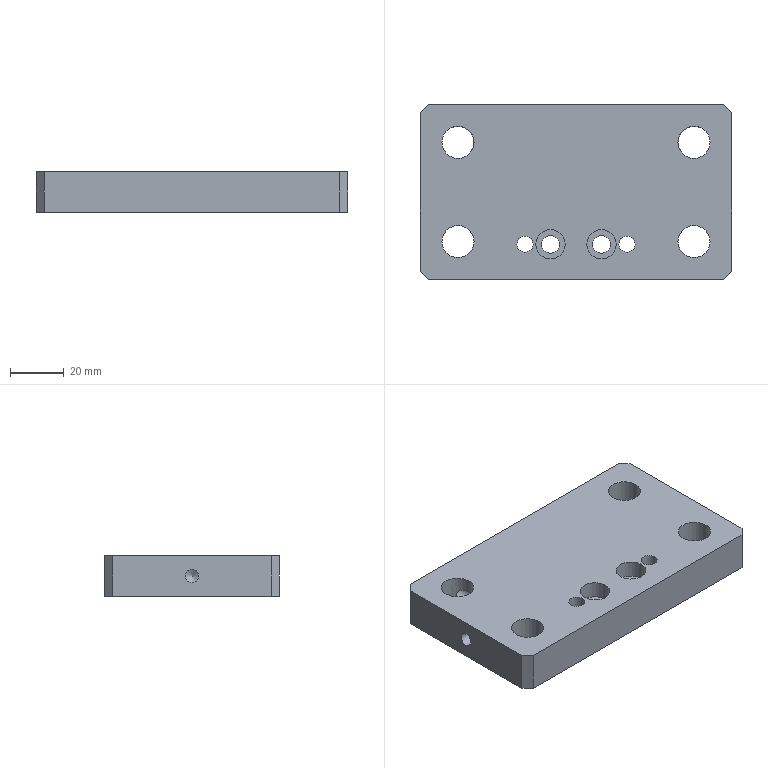Part | NX | features BREP 1 | 1 solid | 31 faces | box 116 x 65 x 15 mm | volume 102234 mm3 | cylinder 15 | plane 12 | cone 4 | commonest cylinder face diameters 5 x5 12 x4 6 x2 6.6 x2 11 x2
STEP:
#1=CARTESIAN_POINT('',(55.,-32.5,0.));
#2=VERTEX_POINT('',#1);
#3=CARTESIAN_POINT('',(58.,-29.5,0.));
#4=VERTEX_POINT('',#3);
#5=CARTESIAN_POINT('',(55.,-32.5,0.));
#6=DIRECTION('',(0.7071,0.7071,0.));
#7=VECTOR('',#6,1000.);
#8=LINE('',#5,#7);
#9=EDGE_CURVE('',#2,#4,#8,.T.);
#10=ORIENTED_EDGE('',*,*,#9,.F.);
#11=CARTESIAN_POINT('',(-55.,-32.5,0.));
#12=VERTEX_POINT('',#11);
#13=CARTESIAN_POINT('',(0.,-32.5,0.));
#14=DIRECTION('',(1.,0.,0.));
#15=VECTOR('',#14,1000.);
#16=LINE('',#13,#15);
#17=EDGE_CURVE('',#12,#2,#16,.T.);
#18=ORIENTED_EDGE('',*,*,#17,.F.);
#19=CARTESIAN_POINT('',(-58.,-29.5,0.));
#20=VERTEX_POINT('',#19);
#21=CARTESIAN_POINT('',(-58.,-29.5,0.));
#22=DIRECTION('',(0.7071,-0.7071,0.));
#23=VECTOR('',#22,1000.);
#24=LINE('',#21,#23);
#25=EDGE_CURVE('',#20,#12,#24,.T.);
#26=ORIENTED_EDGE('',*,*,#25,.F.);
#27=CARTESIAN_POINT('',(-58.,29.5,0.));
#28=VERTEX_POINT('',#27);
#29=CARTESIAN_POINT('',(-58.,0.,0.));
#30=DIRECTION('',(0.,-1.,0.));
#31=VECTOR('',#30,1000.);
#32=LINE('',#29,#31);
#33=EDGE_CURVE('',#28,#20,#32,.T.);
#34=ORIENTED_EDGE('',*,*,#33,.F.);
#35=CARTESIAN_POINT('',(-55.,32.5,0.));
#36=VERTEX_POINT('',#35);
#37=CARTESIAN_POINT('',(-55.,32.5,0.));
#38=DIRECTION('',(-0.7071,-0.7071,0.));
#39=VECTOR('',#38,1000.);
#40=LINE('',#37,#39);
#41=EDGE_CURVE('',#36,#28,#40,.T.);
#42=ORIENTED_EDGE('',*,*,#41,.F.);
#43=CARTESIAN_POINT('',(55.,32.5,0.));
#44=VERTEX_POINT('',#43);
#45=CARTESIAN_POINT('',(0.,32.5,0.));
#46=DIRECTION('',(-1.,0.,0.));
#47=VECTOR('',#46,1000.);
#48=LINE('',#45,#47);
#49=EDGE_CURVE('',#44,#36,#48,.T.);
#50=ORIENTED_EDGE('',*,*,#49,.F.);
#51=CARTESIAN_POINT('',(58.,29.5,0.));
#52=VERTEX_POINT('',#51);
#53=CARTESIAN_POINT('',(58.,29.5,0.));
#54=DIRECTION('',(-0.7071,0.7071,0.));
#55=VECTOR('',#54,1000.);
#56=LINE('',#53,#55);
#57=EDGE_CURVE('',#52,#44,#56,.T.);
#58=ORIENTED_EDGE('',*,*,#57,.F.);
#59=CARTESIAN_POINT('',(58.,0.,0.));
#60=DIRECTION('',(0.,1.,0.));
#61=VECTOR('',#60,1000.);
#62=LINE('',#59,#61);
#63=EDGE_CURVE('',#4,#52,#62,.T.);
#64=ORIENTED_EDGE('',*,*,#63,.F.);
#65=EDGE_LOOP('',(#10,#18,#26,#34,#42,#50,#58,#64));
#66=FACE_BOUND('',#65,.T.);
#67=CARTESIAN_POINT('',(38.,-18.5,0.));
#68=VERTEX_POINT('',#67);
#69=CARTESIAN_POINT('',(44.,-18.5,0.));
#70=DIRECTION('',(0.,0.,-1.));
#71=DIRECTION('',(-1.,0.,0.));
#72=AXIS2_PLACEMENT_3D('',#69,#70,#71);
#73=CIRCLE('',#72,6.);
#74=EDGE_CURVE('',#68,#68,#73,.T.);
#75=ORIENTED_EDGE('',*,*,#74,.F.);
#76=EDGE_LOOP('',(#75));
#77=FACE_BOUND('',#76,.T.);
#78=CARTESIAN_POINT('',(38.,18.5,0.));
#79=VERTEX_POINT('',#78);
#80=CARTESIAN_POINT('',(44.,18.5,0.));
#81=DIRECTION('',(0.,0.,-1.));
#82=DIRECTION('',(-1.,0.,0.));
#83=AXIS2_PLACEMENT_3D('',#80,#81,#82);
#84=CIRCLE('',#83,6.);
#85=EDGE_CURVE('',#79,#79,#84,.T.);
#86=ORIENTED_EDGE('',*,*,#85,.F.);
#87=EDGE_LOOP('',(#86));
#88=FACE_BOUND('',#87,.T.);
#89=CARTESIAN_POINT('',(-50.,18.5,0.));
#90=VERTEX_POINT('',#89);
#91=CARTESIAN_POINT('',(-44.,18.5,0.));
#92=DIRECTION('',(0.,0.,-1.));
#93=DIRECTION('',(-1.,0.,0.));
#94=AXIS2_PLACEMENT_3D('',#91,#92,#93);
#95=CIRCLE('',#94,6.);
#96=EDGE_CURVE('',#90,#90,#95,.T.);
#97=ORIENTED_EDGE('',*,*,#96,.F.);
#98=EDGE_LOOP('',(#97));
#99=FACE_BOUND('',#98,.T.);
#100=CARTESIAN_POINT('',(-50.,-18.5,0.));
#101=VERTEX_POINT('',#100);
#102=CARTESIAN_POINT('',(-44.,-18.5,0.));
#103=DIRECTION('',(0.,0.,-1.));
#104=DIRECTION('',(-1.,0.,0.));
#105=AXIS2_PLACEMENT_3D('',#102,#103,#104);
#106=CIRCLE('',#105,6.);
#107=EDGE_CURVE('',#101,#101,#106,.T.);
#108=ORIENTED_EDGE('',*,*,#107,.F.);
#109=EDGE_LOOP('',(#108));
#110=FACE_BOUND('',#109,.T.);
#111=CARTESIAN_POINT('',(16.,-19.5,0.));
#112=VERTEX_POINT('',#111);
#113=CARTESIAN_POINT('',(19.,-19.5,0.));
#114=DIRECTION('',(0.,0.,-1.));
#115=DIRECTION('',(-1.,0.,0.));
#116=AXIS2_PLACEMENT_3D('',#113,#114,#115);
#117=CIRCLE('',#116,3.);
#118=EDGE_CURVE('',#112,#112,#117,.T.);
#119=ORIENTED_EDGE('',*,*,#118,.F.);
#120=EDGE_LOOP('',(#119));
#121=FACE_BOUND('',#120,.T.);
#122=CARTESIAN_POINT('',(-22.,-19.5,0.));
#123=VERTEX_POINT('',#122);
#124=CARTESIAN_POINT('',(-19.,-19.5,0.));
#125=DIRECTION('',(0.,0.,-1.));
#126=DIRECTION('',(-1.,0.,0.));
#127=AXIS2_PLACEMENT_3D('',#124,#125,#126);
#128=CIRCLE('',#127,3.);
#129=EDGE_CURVE('',#123,#123,#128,.T.);
#130=ORIENTED_EDGE('',*,*,#129,.F.);
#131=EDGE_LOOP('',(#130));
#132=FACE_BOUND('',#131,.T.);
#133=CARTESIAN_POINT('',(12.8,-19.5,0.));
#134=VERTEX_POINT('',#133);
#135=CARTESIAN_POINT('',(9.5,-19.5,0.));
#136=DIRECTION('',(0.,0.,-1.));
#137=DIRECTION('',(1.,0.,0.));
#138=AXIS2_PLACEMENT_3D('',#135,#136,#137);
#139=CIRCLE('',#138,3.3);
#140=EDGE_CURVE('',#134,#134,#139,.T.);
#141=ORIENTED_EDGE('',*,*,#140,.F.);
#142=EDGE_LOOP('',(#141));
#143=FACE_BOUND('',#142,.T.);
#144=CARTESIAN_POINT('',(-6.2,-19.5,0.));
#145=VERTEX_POINT('',#144);
#146=CARTESIAN_POINT('',(-9.5,-19.5,0.));
#147=DIRECTION('',(0.,0.,-1.));
#148=DIRECTION('',(1.,0.,0.));
#149=AXIS2_PLACEMENT_3D('',#146,#147,#148);
#150=CIRCLE('',#149,3.3);
#151=EDGE_CURVE('',#145,#145,#150,.T.);
#152=ORIENTED_EDGE('',*,*,#151,.F.);
#153=EDGE_LOOP('',(#152));
#154=FACE_BOUND('',#153,.T.);
#155=CARTESIAN_POINT('',(0.,0.,0.));
#156=DIRECTION('',(0.,0.,1.));
#157=DIRECTION('',(-1.,0.,0.));
#158=AXIS2_PLACEMENT_3D('',#155,#156,#157);
#159=PLANE('',#158);
#160=ADVANCED_FACE('',(#66,#77,#88,#99,#110,#121,#132,#143,#154),#159,.F.);
#161=CARTESIAN_POINT('',(58.,-29.5,15.));
#162=VERTEX_POINT('',#161);
#163=CARTESIAN_POINT('',(58.,-29.5,15.));
#164=DIRECTION('',(0.,0.,1.));
#165=VECTOR('',#164,1000.);
#166=LINE('',#163,#165);
#167=EDGE_CURVE('',#4,#162,#166,.T.);
#168=ORIENTED_EDGE('',*,*,#167,.F.);
#169=ORIENTED_EDGE('',*,*,#63,.T.);
#170=CARTESIAN_POINT('',(58.,29.5,15.));
#171=VERTEX_POINT('',#170);
#172=CARTESIAN_POINT('',(58.,29.5,15.));
#173=DIRECTION('',(0.,0.,-1.));
#174=VECTOR('',#173,1000.);
#175=LINE('',#172,#174);
#176=EDGE_CURVE('',#171,#52,#175,.T.);
#177=ORIENTED_EDGE('',*,*,#176,.F.);
#178=CARTESIAN_POINT('',(58.,32.5,15.));
#179=DIRECTION('',(0.,1.,0.));
#180=VECTOR('',#179,1000.);
#181=LINE('',#178,#180);
#182=EDGE_CURVE('',#162,#171,#181,.T.);
#183=ORIENTED_EDGE('',*,*,#182,.F.);
#184=EDGE_LOOP('',(#168,#169,#177,#183));
#185=FACE_BOUND('',#184,.T.);
#186=CARTESIAN_POINT('',(58.,0.,5.));
#187=VERTEX_POINT('',#186);
#188=CARTESIAN_POINT('',(58.,0.,7.5));
#189=DIRECTION('',(1.,0.,0.));
#190=DIRECTION('',(0.,0.,-1.));
#191=AXIS2_PLACEMENT_3D('',#188,#189,#190);
#192=CIRCLE('',#191,2.5);
#193=EDGE_CURVE('',#187,#187,#192,.T.);
#194=ORIENTED_EDGE('',*,*,#193,.F.);
#195=EDGE_LOOP('',(#194));
#196=FACE_BOUND('',#195,.T.);
#197=CARTESIAN_POINT('',(58.,32.5,15.));
#198=DIRECTION('',(-1.,0.,0.));
#199=DIRECTION('',(0.,1.,0.));
#200=AXIS2_PLACEMENT_3D('',#197,#198,#199);
#201=PLANE('',#200);
#202=ADVANCED_FACE('',(#185,#196),#201,.F.);
#203=CARTESIAN_POINT('',(55.,-32.5,15.));
#204=VERTEX_POINT('',#203);
#205=CARTESIAN_POINT('',(55.,-32.5,15.));
#206=DIRECTION('',(0.,0.,1.));
#207=VECTOR('',#206,1000.);
#208=LINE('',#205,#207);
#209=EDGE_CURVE('',#2,#204,#208,.T.);
#210=ORIENTED_EDGE('',*,*,#209,.F.);
#211=ORIENTED_EDGE('',*,*,#9,.T.);
#212=ORIENTED_EDGE('',*,*,#167,.T.);
#213=CARTESIAN_POINT('',(58.,-29.5,15.));
#214=DIRECTION('',(0.7071,0.7071,0.));
#215=VECTOR('',#214,1000.);
#216=LINE('',#213,#215);
#217=EDGE_CURVE('',#204,#162,#216,.T.);
#218=ORIENTED_EDGE('',*,*,#217,.F.);
#219=EDGE_LOOP('',(#210,#211,#212,#218));
#220=FACE_BOUND('',#219,.T.);
#221=CARTESIAN_POINT('',(58.,-29.5,15.));
#222=DIRECTION('',(-0.7071,0.7071,0.));
#223=DIRECTION('',(0.7071,0.7071,0.));
#224=AXIS2_PLACEMENT_3D('',#221,#222,#223);
#225=PLANE('',#224);
#226=ADVANCED_FACE('',(#220),#225,.F.);
#227=ORIENTED_EDGE('',*,*,#209,.T.);
#228=CARTESIAN_POINT('',(-55.,-32.5,15.));
#229=VERTEX_POINT('',#228);
#230=CARTESIAN_POINT('',(-58.,-32.5,15.));
#231=DIRECTION('',(1.,0.,0.));
#232=VECTOR('',#231,1000.);
#233=LINE('',#230,#232);
#234=EDGE_CURVE('',#229,#204,#233,.T.);
#235=ORIENTED_EDGE('',*,*,#234,.F.);
#236=CARTESIAN_POINT('',(-55.,-32.5,15.));
#237=DIRECTION('',(0.,0.,1.));
#238=VECTOR('',#237,1000.);
#239=LINE('',#236,#238);
#240=EDGE_CURVE('',#12,#229,#239,.T.);
#241=ORIENTED_EDGE('',*,*,#240,.F.);
#242=ORIENTED_EDGE('',*,*,#17,.T.);
#243=EDGE_LOOP('',(#227,#235,#241,#242));
#244=FACE_BOUND('',#243,.T.);
#245=CARTESIAN_POINT('',(-58.,-32.5,15.));
#246=DIRECTION('',(0.,1.,0.));
#247=DIRECTION('',(0.,0.,-1.));
#248=AXIS2_PLACEMENT_3D('',#245,#246,#247);
#249=PLANE('',#248);
#250=ADVANCED_FACE('',(#244),#249,.F.);
#251=CARTESIAN_POINT('',(-58.,-29.5,15.));
#252=VERTEX_POINT('',#251);
#253=CARTESIAN_POINT('',(-58.,-29.5,15.));
#254=DIRECTION('',(0.,0.,1.));
#255=VECTOR('',#254,1000.);
#256=LINE('',#253,#255);
#257=EDGE_CURVE('',#20,#252,#256,.T.);
#258=ORIENTED_EDGE('',*,*,#257,.F.);
#259=ORIENTED_EDGE('',*,*,#25,.T.);
#260=ORIENTED_EDGE('',*,*,#240,.T.);
#261=CARTESIAN_POINT('',(-55.,-32.5,15.));
#262=DIRECTION('',(0.7071,-0.7071,0.));
#263=VECTOR('',#262,1000.);
#264=LINE('',#261,#263);
#265=EDGE_CURVE('',#252,#229,#264,.T.);
#266=ORIENTED_EDGE('',*,*,#265,.F.);
#267=EDGE_LOOP('',(#258,#259,#260,#266));
#268=FACE_BOUND('',#267,.T.);
#269=CARTESIAN_POINT('',(-55.,-32.5,15.));
#270=DIRECTION('',(0.7071,0.7071,0.));
#271=DIRECTION('',(0.7071,-0.7071,0.));
#272=AXIS2_PLACEMENT_3D('',#269,#270,#271);
#273=PLANE('',#272);
#274=ADVANCED_FACE('',(#268),#273,.F.);
#275=ORIENTED_EDGE('',*,*,#257,.T.);
#276=CARTESIAN_POINT('',(-58.,29.5,15.));
#277=VERTEX_POINT('',#276);
#278=CARTESIAN_POINT('',(-58.,32.5,15.));
#279=DIRECTION('',(0.,-1.,0.));
#280=VECTOR('',#279,1000.);
#281=LINE('',#278,#280);
#282=EDGE_CURVE('',#277,#252,#281,.T.);
#283=ORIENTED_EDGE('',*,*,#282,.F.);
#284=CARTESIAN_POINT('',(-58.,29.5,15.));
#285=DIRECTION('',(0.,0.,1.));
#286=VECTOR('',#285,1000.);
#287=LINE('',#284,#286);
#288=EDGE_CURVE('',#28,#277,#287,.T.);
#289=ORIENTED_EDGE('',*,*,#288,.F.);
#290=ORIENTED_EDGE('',*,*,#33,.T.);
#291=EDGE_LOOP('',(#275,#283,#289,#290));
#292=FACE_BOUND('',#291,.T.);
#293=CARTESIAN_POINT('',(-58.,0.,10.));
#294=VERTEX_POINT('',#293);
#295=CARTESIAN_POINT('',(-58.,0.,7.5));
#296=DIRECTION('',(-1.,0.,0.));
#297=DIRECTION('',(0.,0.,1.));
#298=AXIS2_PLACEMENT_3D('',#295,#296,#297);
#299=CIRCLE('',#298,2.5);
#300=EDGE_CURVE('',#294,#294,#299,.T.);
#301=ORIENTED_EDGE('',*,*,#300,.F.);
#302=EDGE_LOOP('',(#301));
#303=FACE_BOUND('',#302,.T.);
#304=CARTESIAN_POINT('',(-58.,32.5,15.));
#305=DIRECTION('',(1.,0.,0.));
#306=DIRECTION('',(0.,-1.,0.));
#307=AXIS2_PLACEMENT_3D('',#304,#305,#306);
#308=PLANE('',#307);
#309=ADVANCED_FACE('',(#292,#303),#308,.F.);
#310=CARTESIAN_POINT('',(-55.,32.5,15.));
#311=VERTEX_POINT('',#310);
#312=CARTESIAN_POINT('',(-55.,32.5,15.));
#313=DIRECTION('',(0.,0.,1.));
#314=VECTOR('',#313,1000.);
#315=LINE('',#312,#314);
#316=EDGE_CURVE('',#36,#311,#315,.T.);
#317=ORIENTED_EDGE('',*,*,#316,.F.);
#318=ORIENTED_EDGE('',*,*,#41,.T.);
#319=ORIENTED_EDGE('',*,*,#288,.T.);
#320=CARTESIAN_POINT('',(-58.,29.5,15.));
#321=DIRECTION('',(-0.7071,-0.7071,0.));
#322=VECTOR('',#321,1000.);
#323=LINE('',#320,#322);
#324=EDGE_CURVE('',#311,#277,#323,.T.);
#325=ORIENTED_EDGE('',*,*,#324,.F.);
#326=EDGE_LOOP('',(#317,#318,#319,#325));
#327=FACE_BOUND('',#326,.T.);
#328=CARTESIAN_POINT('',(-58.,29.5,15.));
#329=DIRECTION('',(0.7071,-0.7071,0.));
#330=DIRECTION('',(-0.7071,-0.7071,0.));
#331=AXIS2_PLACEMENT_3D('',#328,#329,#330);
#332=PLANE('',#331);
#333=ADVANCED_FACE('',(#327),#332,.F.);
#334=CARTESIAN_POINT('',(55.,32.5,15.));
#335=VERTEX_POINT('',#334);
#336=CARTESIAN_POINT('',(55.,32.5,15.));
#337=DIRECTION('',(0.,0.,1.));
#338=VECTOR('',#337,1000.);
#339=LINE('',#336,#338);
#340=EDGE_CURVE('',#44,#335,#339,.T.);
#341=ORIENTED_EDGE('',*,*,#340,.F.);
#342=ORIENTED_EDGE('',*,*,#49,.T.);
#343=ORIENTED_EDGE('',*,*,#316,.T.);
#344=CARTESIAN_POINT('',(-58.,32.5,15.));
#345=DIRECTION('',(-1.,0.,0.));
#346=VECTOR('',#345,1000.);
#347=LINE('',#344,#346);
#348=EDGE_CURVE('',#335,#311,#347,.T.);
#349=ORIENTED_EDGE('',*,*,#348,.F.);
#350=EDGE_LOOP('',(#341,#342,#343,#349));
#351=FACE_BOUND('',#350,.T.);
#352=CARTESIAN_POINT('',(37.5,32.5,10.));
#353=VERTEX_POINT('',#352);
#354=CARTESIAN_POINT('',(37.5,32.5,7.5));
#355=DIRECTION('',(0.,1.,0.));
#356=DIRECTION('',(0.,0.,1.));
#357=AXIS2_PLACEMENT_3D('',#354,#355,#356);
#358=CIRCLE('',#357,2.5);
#359=EDGE_CURVE('',#353,#353,#358,.T.);
#360=ORIENTED_EDGE('',*,*,#359,.F.);
#361=EDGE_LOOP('',(#360));
#362=FACE_BOUND('',#361,.T.);
#363=CARTESIAN_POINT('',(-37.5,32.5,10.));
#364=VERTEX_POINT('',#363);
#365=CARTESIAN_POINT('',(-37.5,32.5,7.5));
#366=DIRECTION('',(0.,1.,0.));
#367=DIRECTION('',(0.,0.,1.));
#368=AXIS2_PLACEMENT_3D('',#365,#366,#367);
#369=CIRCLE('',#368,2.5);
#370=EDGE_CURVE('',#364,#364,#369,.T.);
#371=ORIENTED_EDGE('',*,*,#370,.F.);
#372=EDGE_LOOP('',(#371));
#373=FACE_BOUND('',#372,.T.);
#374=CARTESIAN_POINT('',(-58.,32.5,15.));
#375=DIRECTION('',(0.,-1.,0.));
#376=DIRECTION('',(0.,0.,1.));
#377=AXIS2_PLACEMENT_3D('',#374,#375,#376);
#378=PLANE('',#377);
#379=ADVANCED_FACE('',(#351,#362,#373),#378,.F.);
#380=ORIENTED_EDGE('',*,*,#176,.T.);
#381=ORIENTED_EDGE('',*,*,#57,.T.);
#382=ORIENTED_EDGE('',*,*,#340,.T.);
#383=CARTESIAN_POINT('',(55.,32.5,15.));
#384=DIRECTION('',(-0.7071,0.7071,0.));
#385=VECTOR('',#384,1000.);
#386=LINE('',#383,#385);
#387=EDGE_CURVE('',#171,#335,#386,.T.);
#388=ORIENTED_EDGE('',*,*,#387,.F.);
#389=EDGE_LOOP('',(#380,#381,#382,#388));
#390=FACE_BOUND('',#389,.T.);
#391=CARTESIAN_POINT('',(55.,32.5,15.));
#392=DIRECTION('',(-0.7071,-0.7071,0.));
#393=DIRECTION('',(-0.7071,0.7071,0.));
#394=AXIS2_PLACEMENT_3D('',#391,#392,#393);
#395=PLANE('',#394);
#396=ADVANCED_FACE('',(#390),#395,.F.);
#397=CARTESIAN_POINT('',(38.,-18.5,15.));
#398=VERTEX_POINT('',#397);
#399=CARTESIAN_POINT('',(44.,-18.5,15.));
#400=DIRECTION('',(0.,0.,-1.));
#401=DIRECTION('',(-1.,0.,0.));
#402=AXIS2_PLACEMENT_3D('',#399,#400,#401);
#403=CIRCLE('',#402,6.);
#404=EDGE_CURVE('',#398,#398,#403,.T.);
#405=ORIENTED_EDGE('',*,*,#404,.F.);
#406=EDGE_LOOP('',(#405));
#407=FACE_BOUND('',#406,.T.);
#408=ORIENTED_EDGE('',*,*,#74,.T.);
#409=EDGE_LOOP('',(#408));
#410=FACE_BOUND('',#409,.T.);
#411=CARTESIAN_POINT('',(44.,-18.5,0.));
#412=DIRECTION('',(0.,0.,-1.));
#413=DIRECTION('',(1.,0.,0.));
#414=AXIS2_PLACEMENT_3D('',#411,#412,#413);
#415=CYLINDRICAL_SURFACE('',#414,6.);
#416=ADVANCED_FACE('',(#407,#410),#415,.F.);
#417=CARTESIAN_POINT('',(38.084,17.5,5.069));
#418=VERTEX_POINT('',#417);
#419=CARTESIAN_POINT('',(38.084,17.5,9.931));
#420=VERTEX_POINT('',#419);
#421=CARTESIAN_POINT('',(38.084,17.5,5.069));
#422=CARTESIAN_POINT('',(37.983,18.098,5.045));
#423=CARTESIAN_POINT('',(37.966,19.305,5.043));
#424=CARTESIAN_POINT('',(38.461,21.047,5.154));
#425=CARTESIAN_POINT('',(39.481,22.542,5.725));
#426=CARTESIAN_POINT('',(40.257,23.185,7.487));
#427=CARTESIAN_POINT('',(39.492,22.553,9.265));
#428=CARTESIAN_POINT('',(38.471,21.068,9.843));
#429=CARTESIAN_POINT('',(37.966,19.32,9.957));
#430=CARTESIAN_POINT('',(37.983,18.098,9.955));
#431=CARTESIAN_POINT('',(38.084,17.5,9.931));
#432=B_SPLINE_CURVE_WITH_KNOTS('',3,(#421,#422,#423,#424,#425,#426,#427,#428,#429,#430,#431),.UNSPECIFIED.,.F.,.F.,(4,1,1,1,1,1,1,1,4),(0.,0.001794,0.003588,0.005381,0.007175,0.008969,0.01076,0.01256,0.01435),.UNSPECIFIED.);
#433=EDGE_CURVE('',#418,#420,#432,.T.);
#434=ORIENTED_EDGE('',*,*,#433,.F.);
#435=CARTESIAN_POINT('',(38.084,17.5,9.931));
#436=CARTESIAN_POINT('',(38.121,17.28,9.545));
#437=CARTESIAN_POINT('',(38.219,16.853,8.787));
#438=CARTESIAN_POINT('',(38.404,16.329,7.497));
#439=CARTESIAN_POINT('',(38.218,16.855,6.211));
#440=CARTESIAN_POINT('',(38.121,17.281,5.454));
#441=CARTESIAN_POINT('',(38.084,17.5,5.069));
#442=B_SPLINE_CURVE_WITH_KNOTS('',3,(#435,#436,#437,#438,#439,#440,#441),.UNSPECIFIED.,.F.,.F.,(4,1,1,1,4),(0.,0.001335,0.002669,0.004004,0.005339),.UNSPECIFIED.);
#443=EDGE_CURVE('',#420,#418,#442,.T.);
#444=ORIENTED_EDGE('',*,*,#443,.F.);
#445=EDGE_LOOP('',(#434,#444));
#446=FACE_BOUND('',#445,.T.);
#447=CARTESIAN_POINT('',(38.,18.5,15.));
#448=VERTEX_POINT('',#447);
#449=CARTESIAN_POINT('',(44.,18.5,15.));
#450=DIRECTION('',(0.,0.,-1.));
#451=DIRECTION('',(-1.,0.,0.));
#452=AXIS2_PLACEMENT_3D('',#449,#450,#451);
#453=CIRCLE('',#452,6.);
#454=EDGE_CURVE('',#448,#448,#453,.T.);
#455=ORIENTED_EDGE('',*,*,#454,.F.);
#456=EDGE_LOOP('',(#455));
#457=FACE_BOUND('',#456,.T.);
#458=ORIENTED_EDGE('',*,*,#85,.T.);
#459=EDGE_LOOP('',(#458));
#460=FACE_BOUND('',#459,.T.);
#461=CARTESIAN_POINT('',(44.,18.5,0.));
#462=DIRECTION('',(0.,0.,-1.));
#463=DIRECTION('',(1.,0.,0.));
#464=AXIS2_PLACEMENT_3D('',#461,#462,#463);
#465=CYLINDRICAL_SURFACE('',#464,6.);
#466=ADVANCED_FACE('',(#446,#457,#460),#465,.F.);
#467=ORIENTED_EDGE('',*,*,#96,.T.);
#468=EDGE_LOOP('',(#467));
#469=FACE_BOUND('',#468,.T.);
#470=CARTESIAN_POINT('',(-50.,18.5,15.));
#471=VERTEX_POINT('',#470);
#472=CARTESIAN_POINT('',(-44.,18.5,15.));
#473=DIRECTION('',(0.,0.,-1.));
#474=DIRECTION('',(-1.,0.,0.));
#475=AXIS2_PLACEMENT_3D('',#472,#473,#474);
#476=CIRCLE('',#475,6.);
#477=EDGE_CURVE('',#471,#471,#476,.T.);
#478=ORIENTED_EDGE('',*,*,#477,.F.);
#479=EDGE_LOOP('',(#478));
#480=FACE_BOUND('',#479,.T.);
#481=CARTESIAN_POINT('',(-38.084,17.5,5.069));
#482=VERTEX_POINT('',#481);
#483=CARTESIAN_POINT('',(-38.084,17.5,9.931));
#484=VERTEX_POINT('',#483);
#485=CARTESIAN_POINT('',(-38.084,17.5,5.069));
#486=CARTESIAN_POINT('',(-38.121,17.28,5.455));
#487=CARTESIAN_POINT('',(-38.219,16.853,6.213));
#488=CARTESIAN_POINT('',(-38.404,16.329,7.503));
#489=CARTESIAN_POINT('',(-38.218,16.855,8.789));
#490=CARTESIAN_POINT('',(-38.121,17.281,9.546));
#491=CARTESIAN_POINT('',(-38.084,17.5,9.931));
#492=B_SPLINE_CURVE_WITH_KNOTS('',3,(#485,#486,#487,#488,#489,#490,#491),.UNSPECIFIED.,.F.,.F.,(4,1,1,1,4),(0.,0.001335,0.002669,0.004004,0.005339),.UNSPECIFIED.);
#493=EDGE_CURVE('',#482,#484,#492,.T.);
#494=ORIENTED_EDGE('',*,*,#493,.F.);
#495=CARTESIAN_POINT('',(-38.084,17.5,9.931));
#496=CARTESIAN_POINT('',(-37.983,18.098,9.955));
#497=CARTESIAN_POINT('',(-37.966,19.305,9.957));
#498=CARTESIAN_POINT('',(-38.461,21.047,9.846));
#499=CARTESIAN_POINT('',(-39.481,22.542,9.275));
#500=CARTESIAN_POINT('',(-40.257,23.185,7.513));
#501=CARTESIAN_POINT('',(-39.492,22.553,5.735));
#502=CARTESIAN_POINT('',(-38.471,21.068,5.157));
#503=CARTESIAN_POINT('',(-37.966,19.32,5.043));
#504=CARTESIAN_POINT('',(-37.983,18.098,5.045));
#505=CARTESIAN_POINT('',(-38.084,17.5,5.069));
#506=B_SPLINE_CURVE_WITH_KNOTS('',3,(#495,#496,#497,#498,#499,#500,#501,#502,#503,#504,#505),.UNSPECIFIED.,.F.,.F.,(4,1,1,1,1,1,1,1,4),(0.,0.001794,0.003588,0.005381,0.007175,0.008969,0.01076,0.01256,0.01435),.UNSPECIFIED.);
#507=EDGE_CURVE('',#484,#482,#506,.T.);
#508=ORIENTED_EDGE('',*,*,#507,.F.);
#509=EDGE_LOOP('',(#494,#508));
#510=FACE_BOUND('',#509,.T.);
#511=CARTESIAN_POINT('',(-44.,18.5,0.));
#512=DIRECTION('',(0.,0.,-1.));
#513=DIRECTION('',(1.,0.,0.));
#514=AXIS2_PLACEMENT_3D('',#511,#512,#513);
#515=CYLINDRICAL_SURFACE('',#514,6.);
#516=ADVANCED_FACE('',(#469,#480,#510),#515,.F.);
#517=CARTESIAN_POINT('',(-50.,-18.5,15.));
#518=VERTEX_POINT('',#517);
#519=CARTESIAN_POINT('',(-44.,-18.5,15.));
#520=DIRECTION('',(0.,0.,-1.));
#521=DIRECTION('',(-1.,0.,0.));
#522=AXIS2_PLACEMENT_3D('',#519,#520,#521);
#523=CIRCLE('',#522,6.);
#524=EDGE_CURVE('',#518,#518,#523,.T.);
#525=ORIENTED_EDGE('',*,*,#524,.F.);
#526=EDGE_LOOP('',(#525));
#527=FACE_BOUND('',#526,.T.);
#528=ORIENTED_EDGE('',*,*,#107,.T.);
#529=EDGE_LOOP('',(#528));
#530=FACE_BOUND('',#529,.T.);
#531=CARTESIAN_POINT('',(-44.,-18.5,0.));
#532=DIRECTION('',(0.,0.,-1.));
#533=DIRECTION('',(1.,0.,0.));
#534=AXIS2_PLACEMENT_3D('',#531,#532,#533);
#535=CYLINDRICAL_SURFACE('',#534,6.);
#536=ADVANCED_FACE('',(#527,#530),#535,.F.);
#537=CARTESIAN_POINT('',(16.,-19.5,15.));
#538=VERTEX_POINT('',#537);
#539=CARTESIAN_POINT('',(19.,-19.5,15.));
#540=DIRECTION('',(0.,0.,-1.));
#541=DIRECTION('',(-1.,0.,0.));
#542=AXIS2_PLACEMENT_3D('',#539,#540,#541);
#543=CIRCLE('',#542,3.);
#544=EDGE_CURVE('',#538,#538,#543,.T.);
#545=ORIENTED_EDGE('',*,*,#544,.F.);
#546=EDGE_LOOP('',(#545));
#547=FACE_BOUND('',#546,.T.);
#548=ORIENTED_EDGE('',*,*,#118,.T.);
#549=EDGE_LOOP('',(#548));
#550=FACE_BOUND('',#549,.T.);
#551=CARTESIAN_POINT('',(19.,-19.5,0.));
#552=DIRECTION('',(0.,0.,-1.));
#553=DIRECTION('',(1.,0.,0.));
#554=AXIS2_PLACEMENT_3D('',#551,#552,#553);
#555=CYLINDRICAL_SURFACE('',#554,3.);
#556=ADVANCED_FACE('',(#547,#550),#555,.F.);
#557=CARTESIAN_POINT('',(-22.,-19.5,15.));
#558=VERTEX_POINT('',#557);
#559=CARTESIAN_POINT('',(-19.,-19.5,15.));
#560=DIRECTION('',(0.,0.,-1.));
#561=DIRECTION('',(-1.,0.,0.));
#562=AXIS2_PLACEMENT_3D('',#559,#560,#561);
#563=CIRCLE('',#562,3.);
#564=EDGE_CURVE('',#558,#558,#563,.T.);
#565=ORIENTED_EDGE('',*,*,#564,.F.);
#566=EDGE_LOOP('',(#565));
#567=FACE_BOUND('',#566,.T.);
#568=ORIENTED_EDGE('',*,*,#129,.T.);
#569=EDGE_LOOP('',(#568));
#570=FACE_BOUND('',#569,.T.);
#571=CARTESIAN_POINT('',(-19.,-19.5,0.));
#572=DIRECTION('',(0.,0.,-1.));
#573=DIRECTION('',(1.,0.,0.));
#574=AXIS2_PLACEMENT_3D('',#571,#572,#573);
#575=CYLINDRICAL_SURFACE('',#574,3.);
#576=ADVANCED_FACE('',(#567,#570),#575,.F.);
#577=ORIENTED_EDGE('',*,*,#140,.T.);
#578=EDGE_LOOP('',(#577));
#579=FACE_BOUND('',#578,.T.);
#580=CARTESIAN_POINT('',(12.8,-19.5,8.6));
#581=VERTEX_POINT('',#580);
#582=CARTESIAN_POINT('',(9.5,-19.5,8.6));
#583=DIRECTION('',(0.,0.,-1.));
#584=DIRECTION('',(1.,0.,0.));
#585=AXIS2_PLACEMENT_3D('',#582,#583,#584);
#586=CIRCLE('',#585,3.3);
#587=EDGE_CURVE('',#581,#581,#586,.T.);
#588=ORIENTED_EDGE('',*,*,#587,.F.);
#589=EDGE_LOOP('',(#588));
#590=FACE_BOUND('',#589,.T.);
#591=CARTESIAN_POINT('',(9.5,-19.5,15.));
#592=DIRECTION('',(0.,0.,1.));
#593=DIRECTION('',(-1.,0.,0.));
#594=AXIS2_PLACEMENT_3D('',#591,#592,#593);
#595=CYLINDRICAL_SURFACE('',#594,3.3);
#596=ADVANCED_FACE('',(#579,#590),#595,.F.);
#597=ORIENTED_EDGE('',*,*,#151,.T.);
#598=EDGE_LOOP('',(#597));
#599=FACE_BOUND('',#598,.T.);
#600=CARTESIAN_POINT('',(-6.2,-19.5,8.6));
#601=VERTEX_POINT('',#600);
#602=CARTESIAN_POINT('',(-9.5,-19.5,8.6));
#603=DIRECTION('',(0.,0.,-1.));
#604=DIRECTION('',(1.,0.,0.));
#605=AXIS2_PLACEMENT_3D('',#602,#603,#604);
#606=CIRCLE('',#605,3.3);
#607=EDGE_CURVE('',#601,#601,#606,.T.);
#608=ORIENTED_EDGE('',*,*,#607,.F.);
#609=EDGE_LOOP('',(#608));
#610=FACE_BOUND('',#609,.T.);
#611=CARTESIAN_POINT('',(-9.5,-19.5,15.));
#612=DIRECTION('',(0.,0.,1.));
#613=DIRECTION('',(-1.,0.,0.));
#614=AXIS2_PLACEMENT_3D('',#611,#612,#613);
#615=CYLINDRICAL_SURFACE('',#614,3.3);
#616=ADVANCED_FACE('',(#599,#610),#615,.F.);
#617=ORIENTED_EDGE('',*,*,#282,.T.);
#618=ORIENTED_EDGE('',*,*,#265,.T.);
#619=ORIENTED_EDGE('',*,*,#234,.T.);
#620=ORIENTED_EDGE('',*,*,#217,.T.);
#621=ORIENTED_EDGE('',*,*,#182,.T.);
#622=ORIENTED_EDGE('',*,*,#387,.T.);
#623=ORIENTED_EDGE('',*,*,#348,.T.);
#624=ORIENTED_EDGE('',*,*,#324,.T.);
#625=EDGE_LOOP('',(#617,#618,#619,#620,#621,#622,#623,#624));
#626=FACE_BOUND('',#625,.T.);
#627=ORIENTED_EDGE('',*,*,#404,.T.);
#628=EDGE_LOOP('',(#627));
#629=FACE_BOUND('',#628,.T.);
#630=ORIENTED_EDGE('',*,*,#454,.T.);
#631=EDGE_LOOP('',(#630));
#632=FACE_BOUND('',#631,.T.);
#633=ORIENTED_EDGE('',*,*,#477,.T.);
#634=EDGE_LOOP('',(#633));
#635=FACE_BOUND('',#634,.T.);
#636=ORIENTED_EDGE('',*,*,#524,.T.);
#637=EDGE_LOOP('',(#636));
#638=FACE_BOUND('',#637,.T.);
#639=ORIENTED_EDGE('',*,*,#544,.T.);
#640=EDGE_LOOP('',(#639));
#641=FACE_BOUND('',#640,.T.);
#642=ORIENTED_EDGE('',*,*,#564,.T.);
#643=EDGE_LOOP('',(#642));
#644=FACE_BOUND('',#643,.T.);
#645=CARTESIAN_POINT('',(15.,-19.5,15.));
#646=VERTEX_POINT('',#645);
#647=CARTESIAN_POINT('',(9.5,-19.5,15.));
#648=DIRECTION('',(0.,0.,-1.));
#649=DIRECTION('',(1.,0.,0.));
#650=AXIS2_PLACEMENT_3D('',#647,#648,#649);
#651=CIRCLE('',#650,5.5);
#652=EDGE_CURVE('',#646,#646,#651,.T.);
#653=ORIENTED_EDGE('',*,*,#652,.T.);
#654=EDGE_LOOP('',(#653));
#655=FACE_BOUND('',#654,.T.);
#656=CARTESIAN_POINT('',(-4.,-19.5,15.));
#657=VERTEX_POINT('',#656);
#658=CARTESIAN_POINT('',(-9.5,-19.5,15.));
#659=DIRECTION('',(0.,0.,-1.));
#660=DIRECTION('',(1.,0.,0.));
#661=AXIS2_PLACEMENT_3D('',#658,#659,#660);
#662=CIRCLE('',#661,5.5);
#663=EDGE_CURVE('',#657,#657,#662,.T.);
#664=ORIENTED_EDGE('',*,*,#663,.T.);
#665=EDGE_LOOP('',(#664));
#666=FACE_BOUND('',#665,.T.);
#667=CARTESIAN_POINT('',(0.,0.,15.));
#668=DIRECTION('',(0.,0.,1.));
#669=DIRECTION('',(-1.,0.,0.));
#670=AXIS2_PLACEMENT_3D('',#667,#668,#669);
#671=PLANE('',#670);
#672=ADVANCED_FACE('',(#626,#629,#632,#635,#638,#641,#644,#655,#666),#671,.T.);
#673=CARTESIAN_POINT('',(43.,0.,5.));
#674=VERTEX_POINT('',#673);
#675=CARTESIAN_POINT('',(43.,0.,7.5));
#676=DIRECTION('',(1.,0.,0.));
#677=DIRECTION('',(0.,0.,-1.));
#678=AXIS2_PLACEMENT_3D('',#675,#676,#677);
#679=CIRCLE('',#678,2.5);
#680=EDGE_CURVE('',#674,#674,#679,.T.);
#681=ORIENTED_EDGE('',*,*,#680,.F.);
#682=EDGE_LOOP('',(#681));
#683=FACE_BOUND('',#682,.T.);
#684=ORIENTED_EDGE('',*,*,#193,.T.);
#685=EDGE_LOOP('',(#684));
#686=FACE_BOUND('',#685,.T.);
#687=CARTESIAN_POINT('',(58.,0.,7.5));
#688=DIRECTION('',(1.,0.,0.));
#689=DIRECTION('',(0.,0.,1.));
#690=AXIS2_PLACEMENT_3D('',#687,#688,#689);
#691=CYLINDRICAL_SURFACE('',#690,2.5);
#692=ADVANCED_FACE('',(#683,#686),#691,.F.);
#693=CARTESIAN_POINT('',(-43.,0.,10.));
#694=VERTEX_POINT('',#693);
#695=CARTESIAN_POINT('',(-43.,0.,7.5));
#696=DIRECTION('',(-1.,0.,0.));
#697=DIRECTION('',(0.,0.,1.));
#698=AXIS2_PLACEMENT_3D('',#695,#696,#697);
#699=CIRCLE('',#698,2.5);
#700=EDGE_CURVE('',#694,#694,#699,.T.);
#701=ORIENTED_EDGE('',*,*,#700,.F.);
#702=EDGE_LOOP('',(#701));
#703=FACE_BOUND('',#702,.T.);
#704=ORIENTED_EDGE('',*,*,#300,.T.);
#705=EDGE_LOOP('',(#704));
#706=FACE_BOUND('',#705,.T.);
#707=CARTESIAN_POINT('',(-58.,0.,7.5));
#708=DIRECTION('',(-1.,0.,0.));
#709=DIRECTION('',(0.,0.,-1.));
#710=AXIS2_PLACEMENT_3D('',#707,#708,#709);
#711=CYLINDRICAL_SURFACE('',#710,2.5);
#712=ADVANCED_FACE('',(#703,#706),#711,.F.);
#713=ORIENTED_EDGE('',*,*,#433,.T.);
#714=CARTESIAN_POINT('',(37.5,17.5,7.5));
#715=DIRECTION('',(0.,1.,0.));
#716=DIRECTION('',(0.,0.,1.));
#717=AXIS2_PLACEMENT_3D('',#714,#715,#716);
#718=CIRCLE('',#717,2.5);
#719=EDGE_CURVE('',#418,#420,#718,.T.);
#720=ORIENTED_EDGE('',*,*,#719,.F.);
#721=EDGE_LOOP('',(#713,#720));
#722=FACE_BOUND('',#721,.T.);
#723=ORIENTED_EDGE('',*,*,#359,.T.);
#724=EDGE_LOOP('',(#723));
#725=FACE_BOUND('',#724,.T.);
#726=CARTESIAN_POINT('',(37.5,32.5,7.5));
#727=DIRECTION('',(0.,1.,0.));
#728=DIRECTION('',(0.,0.,-1.));
#729=AXIS2_PLACEMENT_3D('',#726,#727,#728);
#730=CYLINDRICAL_SURFACE('',#729,2.5);
#731=ADVANCED_FACE('',(#722,#725),#730,.F.);
#732=CARTESIAN_POINT('',(-37.5,17.5,7.5));
#733=DIRECTION('',(0.,1.,0.));
#734=DIRECTION('',(0.,0.,1.));
#735=AXIS2_PLACEMENT_3D('',#732,#733,#734);
#736=CIRCLE('',#735,2.5);
#737=EDGE_CURVE('',#484,#482,#736,.T.);
#738=ORIENTED_EDGE('',*,*,#737,.F.);
#739=ORIENTED_EDGE('',*,*,#507,.T.);
#740=EDGE_LOOP('',(#738,#739));
#741=FACE_BOUND('',#740,.T.);
#742=ORIENTED_EDGE('',*,*,#370,.T.);
#743=EDGE_LOOP('',(#742));
#744=FACE_BOUND('',#743,.T.);
#745=CARTESIAN_POINT('',(-37.5,32.5,7.5));
#746=DIRECTION('',(0.,1.,0.));
#747=DIRECTION('',(0.,0.,-1.));
#748=AXIS2_PLACEMENT_3D('',#745,#746,#747);
#749=CYLINDRICAL_SURFACE('',#748,2.5);
#750=ADVANCED_FACE('',(#741,#744),#749,.F.);
#751=ORIENTED_EDGE('',*,*,#719,.T.);
#752=ORIENTED_EDGE('',*,*,#443,.T.);
#753=EDGE_LOOP('',(#751,#752));
#754=FACE_BOUND('',#753,.T.);
#755=CARTESIAN_POINT('',(37.5,17.5,7.5));
#756=DIRECTION('',(0.,1.,0.));
#757=DIRECTION('',(0.,0.,-1.));
#758=AXIS2_PLACEMENT_3D('',#755,#756,#757);
#759=CONICAL_SURFACE('',#758,2.5,1.03);
#760=ADVANCED_FACE('',(#754),#759,.F.);
#761=ORIENTED_EDGE('',*,*,#737,.T.);
#762=ORIENTED_EDGE('',*,*,#493,.T.);
#763=EDGE_LOOP('',(#761,#762));
#764=FACE_BOUND('',#763,.T.);
#765=CARTESIAN_POINT('',(-37.5,17.5,7.5));
#766=DIRECTION('',(0.,1.,0.));
#767=DIRECTION('',(0.,0.,-1.));
#768=AXIS2_PLACEMENT_3D('',#765,#766,#767);
#769=CONICAL_SURFACE('',#768,2.5,1.03);
#770=ADVANCED_FACE('',(#764),#769,.F.);
#771=CARTESIAN_POINT('',(15.,-19.5,8.6));
#772=VERTEX_POINT('',#771);
#773=CARTESIAN_POINT('',(9.5,-19.5,8.6));
#774=DIRECTION('',(0.,0.,-1.));
#775=DIRECTION('',(1.,0.,0.));
#776=AXIS2_PLACEMENT_3D('',#773,#774,#775);
#777=CIRCLE('',#776,5.5);
#778=EDGE_CURVE('',#772,#772,#777,.T.);
#779=ORIENTED_EDGE('',*,*,#778,.F.);
#780=EDGE_LOOP('',(#779));
#781=FACE_BOUND('',#780,.T.);
#782=ORIENTED_EDGE('',*,*,#587,.T.);
#783=EDGE_LOOP('',(#782));
#784=FACE_BOUND('',#783,.T.);
#785=CARTESIAN_POINT('',(12.8,-19.5,8.6));
#786=DIRECTION('',(0.,0.,-1.));
#787=DIRECTION('',(1.,0.,0.));
#788=AXIS2_PLACEMENT_3D('',#785,#786,#787);
#789=PLANE('',#788);
#790=ADVANCED_FACE('',(#781,#784),#789,.F.);
#791=CARTESIAN_POINT('',(-4.,-19.5,8.6));
#792=VERTEX_POINT('',#791);
#793=CARTESIAN_POINT('',(-9.5,-19.5,8.6));
#794=DIRECTION('',(0.,0.,-1.));
#795=DIRECTION('',(1.,0.,0.));
#796=AXIS2_PLACEMENT_3D('',#793,#794,#795);
#797=CIRCLE('',#796,5.5);
#798=EDGE_CURVE('',#792,#792,#797,.T.);
#799=ORIENTED_EDGE('',*,*,#798,.F.);
#800=EDGE_LOOP('',(#799));
#801=FACE_BOUND('',#800,.T.);
#802=ORIENTED_EDGE('',*,*,#607,.T.);
#803=EDGE_LOOP('',(#802));
#804=FACE_BOUND('',#803,.T.);
#805=CARTESIAN_POINT('',(-6.2,-19.5,8.6));
#806=DIRECTION('',(0.,0.,-1.));
#807=DIRECTION('',(1.,0.,0.));
#808=AXIS2_PLACEMENT_3D('',#805,#806,#807);
#809=PLANE('',#808);
#810=ADVANCED_FACE('',(#801,#804),#809,.F.);
#811=ORIENTED_EDGE('',*,*,#652,.F.);
#812=EDGE_LOOP('',(#811));
#813=FACE_BOUND('',#812,.T.);
#814=ORIENTED_EDGE('',*,*,#778,.T.);
#815=EDGE_LOOP('',(#814));
#816=FACE_BOUND('',#815,.T.);
#817=CARTESIAN_POINT('',(9.5,-19.5,15.));
#818=DIRECTION('',(0.,0.,1.));
#819=DIRECTION('',(-1.,0.,0.));
#820=AXIS2_PLACEMENT_3D('',#817,#818,#819);
#821=CYLINDRICAL_SURFACE('',#820,5.5);
#822=ADVANCED_FACE('',(#813,#816),#821,.F.);
#823=ORIENTED_EDGE('',*,*,#663,.F.);
#824=EDGE_LOOP('',(#823));
#825=FACE_BOUND('',#824,.T.);
#826=ORIENTED_EDGE('',*,*,#798,.T.);
#827=EDGE_LOOP('',(#826));
#828=FACE_BOUND('',#827,.T.);
#829=CARTESIAN_POINT('',(-9.5,-19.5,15.));
#830=DIRECTION('',(0.,0.,1.));
#831=DIRECTION('',(-1.,0.,0.));
#832=AXIS2_PLACEMENT_3D('',#829,#830,#831);
#833=CYLINDRICAL_SURFACE('',#832,5.5);
#834=ADVANCED_FACE('',(#825,#828),#833,.F.);
#835=CARTESIAN_POINT('',(41.498,0.,7.5));
#836=VERTEX_POINT('',#835);
#837=VERTEX_LOOP('',#836);
#838=FACE_BOUND('',#837,.T.);
#839=ORIENTED_EDGE('',*,*,#680,.T.);
#840=EDGE_LOOP('',(#839));
#841=FACE_BOUND('',#840,.T.);
#842=CARTESIAN_POINT('',(43.,0.,7.5));
#843=DIRECTION('',(1.,0.,0.));
#844=DIRECTION('',(0.,0.,1.));
#845=AXIS2_PLACEMENT_3D('',#842,#843,#844);
#846=CONICAL_SURFACE('',#845,2.5,1.03);
#847=ADVANCED_FACE('',(#838,#841),#846,.F.);
#848=CARTESIAN_POINT('',(-41.498,0.,7.5));
#849=VERTEX_POINT('',#848);
#850=VERTEX_LOOP('',#849);
#851=FACE_BOUND('',#850,.T.);
#852=ORIENTED_EDGE('',*,*,#700,.T.);
#853=EDGE_LOOP('',(#852));
#854=FACE_BOUND('',#853,.T.);
#855=CARTESIAN_POINT('',(-43.,0.,7.5));
#856=DIRECTION('',(-1.,0.,0.));
#857=DIRECTION('',(0.,0.,-1.));
#858=AXIS2_PLACEMENT_3D('',#855,#856,#857);
#859=CONICAL_SURFACE('',#858,2.5,1.03);
#860=ADVANCED_FACE('',(#851,#854),#859,.F.);
#861=CLOSED_SHELL('',(#160,#202,#226,#250,#274,#309,#333,#379,#396,#416,#466,#516,#536,#556,#576,#596,#616,#672,#692,#712,#731,#750,#760,#770,#790,#810,#822,#834,#847,#860));
#862=MANIFOLD_SOLID_BREP('',#861);
#863=(LENGTH_UNIT()NAMED_UNIT(*)SI_UNIT(.MILLI.,.METRE.));
#864=UNCERTAINTY_MEASURE_WITH_UNIT(LENGTH_MEASURE(0.0508),#863,'','');
#865=(NAMED_UNIT(*)PLANE_ANGLE_UNIT()SI_UNIT($,.RADIAN.));
#866=(NAMED_UNIT(*)SI_UNIT($,.STERADIAN.)SOLID_ANGLE_UNIT());
#867=(GEOMETRIC_REPRESENTATION_CONTEXT(3)GLOBAL_UNCERTAINTY_ASSIGNED_CONTEXT((#864))GLOBAL_UNIT_ASSIGNED_CONTEXT((#863,#865,#866))REPRESENTATION_CONTEXT('',''));
#868=ADVANCED_BREP_SHAPE_REPRESENTATION('',(#862),#867);